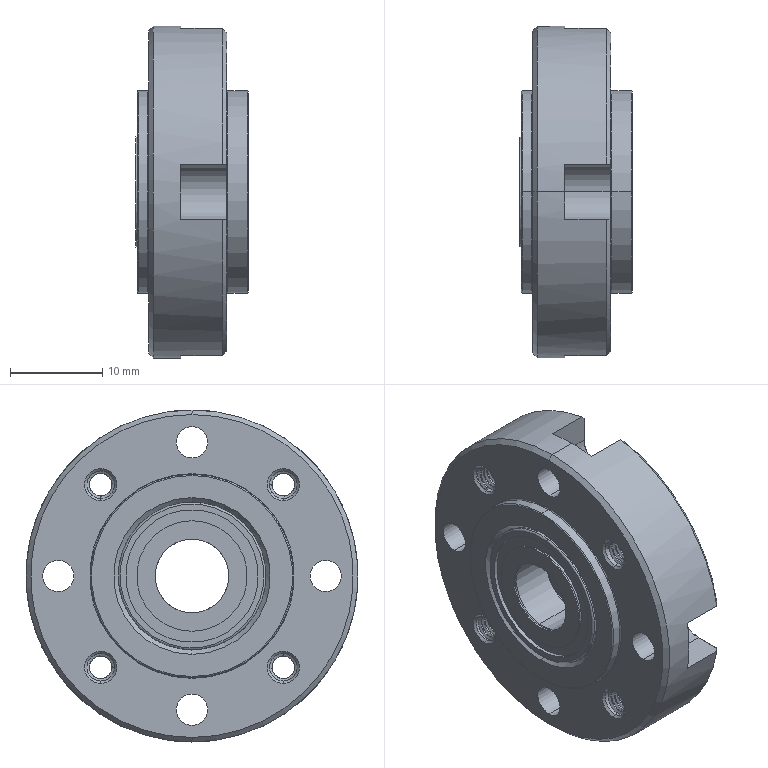Part | SolidWorks | 4 solids | 766 faces | box 12.18 x 36 x 36 mm | volume 7699 mm3 | sphere 312 | cylinder 207 | torus 113 | plane 96 | cone 26 | spline 12 | commonest cylinder face diameters 3 x122 14.4 x16 0.2 x8 3.4 x8 10.8 x8 11.592 x8